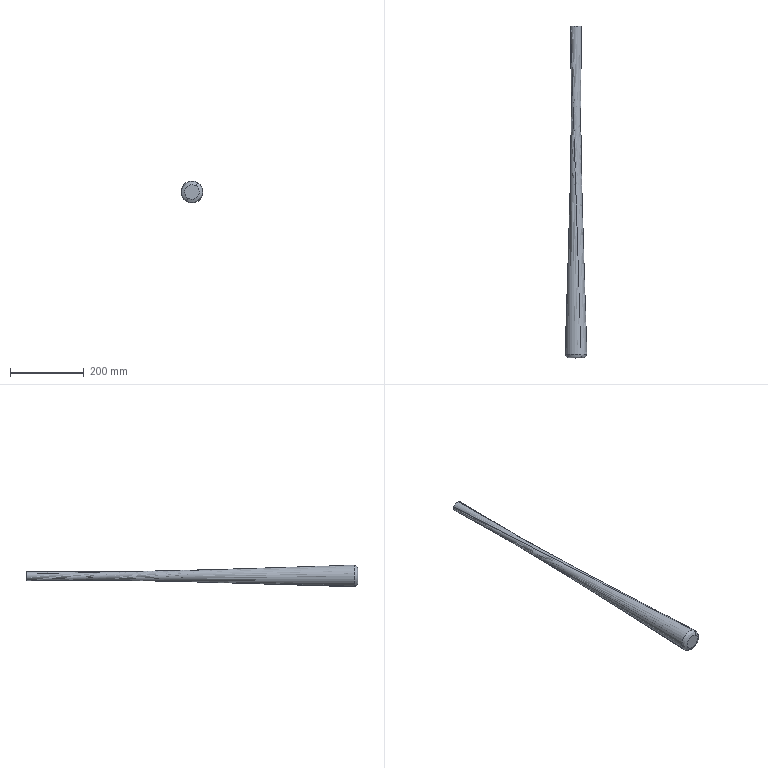Part | SolidWorks | features Blend 1, Fillet 1, RefAxis 1 | 1 solid | 6 faces | box 59.295 x 900 x 59.299 mm | volume 989144 mm3 | spline 4 | plane 2
STEP:
#1=CARTESIAN_POINT('',(-16.101,10.357,-24.873));
#2=VERTEX_POINT('',#1);
#3=CARTESIAN_POINT('',(13.223,10.355,26.518));
#4=VERTEX_POINT('',#3);
#5=CARTESIAN_POINT('',(-16.101,10.357,-24.873));
#6=CARTESIAN_POINT('',(-16.889,10.357,-24.362));
#7=CARTESIAN_POINT('',(-17.653,10.358,-23.815));
#8=CARTESIAN_POINT('',(-19.131,10.358,-22.644));
#9=CARTESIAN_POINT('',(-19.839,10.358,-22.025));
#10=CARTESIAN_POINT('',(-21.861,10.359,-20.085));
#11=CARTESIAN_POINT('',(-23.077,10.359,-18.676));
#12=CARTESIAN_POINT('',(-24.431,10.358,-16.769));
#13=CARTESIAN_POINT('',(-24.694,10.358,-16.38));
#14=CARTESIAN_POINT('',(-25.202,10.358,-15.588));
#15=CARTESIAN_POINT('',(-25.447,10.357,-15.184));
#16=CARTESIAN_POINT('',(-26.151,10.357,-13.963));
#17=CARTESIAN_POINT('',(-26.578,10.356,-13.132));
#18=CARTESIAN_POINT('',(-27.738,10.355,-10.589));
#19=CARTESIAN_POINT('',(-28.35,10.354,-8.829));
#20=CARTESIAN_POINT('',(-28.907,10.352,-6.545));
#21=CARTESIAN_POINT('',(-29.008,10.351,-6.083));
#22=CARTESIAN_POINT('',(-29.188,10.35,-5.16));
#23=CARTESIAN_POINT('',(-29.266,10.35,-4.698));
#24=CARTESIAN_POINT('',(-29.468,10.349,-3.31));
#25=CARTESIAN_POINT('',(-29.648,10.347,-1.456));
#26=CARTESIAN_POINT('',(-29.654,10.345,0.4073));
#27=CARTESIAN_POINT('',(-29.592,10.344,1.808));
#28=CARTESIAN_POINT('',(-29.56,10.344,2.275));
#29=CARTESIAN_POINT('',(-29.474,10.343,3.211));
#30=CARTESIAN_POINT('',(-29.42,10.342,3.681));
#31=CARTESIAN_POINT('',(-29.093,10.34,6.01));
#32=CARTESIAN_POINT('',(-28.659,10.339,7.823));
#33=CARTESIAN_POINT('',(-27.758,10.336,10.468));
#34=CARTESIAN_POINT('',(-27.416,10.336,11.337));
#35=CARTESIAN_POINT('',(-26.837,10.335,12.621));
#36=CARTESIAN_POINT('',(-26.633,10.334,13.047));
#37=CARTESIAN_POINT('',(-26.206,10.334,13.887));
#38=CARTESIAN_POINT('',(-25.983,10.334,14.3));
#39=CARTESIAN_POINT('',(-24.824,10.332,16.332));
#40=CARTESIAN_POINT('',(-23.753,10.332,17.855));
#41=CARTESIAN_POINT('',(-21.933,10.331,19.984));
#42=CARTESIAN_POINT('',(-21.29,10.331,20.669));
#43=CARTESIAN_POINT('',(-19.934,10.331,21.98));
#44=CARTESIAN_POINT('',(-19.23,10.331,22.597));
#45=CARTESIAN_POINT('',(-17.043,10.331,24.342));
#46=CARTESIAN_POINT('',(-15.485,10.332,25.362));
#47=CARTESIAN_POINT('',(-12.996,10.333,26.672));
#48=CARTESIAN_POINT('',(-12.138,10.334,27.073));
#49=CARTESIAN_POINT('',(-10.403,10.335,27.784));
#50=CARTESIAN_POINT('',(-9.524,10.336,28.097));
#51=CARTESIAN_POINT('',(-6.852,10.338,28.908));
#52=CARTESIAN_POINT('',(-5.025,10.339,29.281));
#53=CARTESIAN_POINT('',(-2.211,10.342,29.578));
#54=CARTESIAN_POINT('',(-1.273,10.343,29.632));
#55=CARTESIAN_POINT('',(0.5936,10.344,29.652));
#56=CARTESIAN_POINT('',(1.524,10.345,29.618));
#57=CARTESIAN_POINT('',(3.379,10.347,29.462));
#58=CARTESIAN_POINT('',(4.303,10.348,29.34));
#59=CARTESIAN_POINT('',(6.146,10.35,29.009));
#60=CARTESIAN_POINT('',(7.068,10.35,28.797));
#61=CARTESIAN_POINT('',(9.785,10.353,28.035));
#62=CARTESIAN_POINT('',(11.535,10.354,27.361));
#63=CARTESIAN_POINT('',(13.223,10.355,26.518));
#64=B_SPLINE_CURVE_WITH_KNOTS('',3,(#5,#6,#7,#8,#9,#10,#11,#12,#13,#14,#15,#16,#17,#18,#19,#20,#21,#22,#23,#24,#25,#26,#27,#28,#29,#30,#31,#32,#33,#34,#35,#36,#37,#38,#39,#40,#41,#42,#43,#44,#45,#46,#47,#48,#49,#50,#51,#52,#53,#54,#55,#56,#57,#58,#59,#60,#61,#62,#63),.UNSPECIFIED.,.F.,.F.,(4,2,2,2,2,2,2,2,2,2,1,2,2,2,2,2,2,2,2,2,2,2,2,2,2,2,2,2,2,4),(0.09701,0.09984,0.1027,0.1083,0.1097,0.1112,0.114,0.1196,0.1211,0.1225,0.1253,0.1281,0.1295,0.1309,0.1366,0.1394,0.1408,0.1423,0.1479,0.1507,0.1536,0.1592,0.1621,0.1649,0.1705,0.1734,0.1762,0.179,0.1818,0.1875),.UNSPECIFIED.);
#65=EDGE_CURVE('',#2,#4,#64,.T.);
#66=ORIENTED_EDGE('',*,*,#65,.F.);
#67=CARTESIAN_POINT('',(-10.667,0.,-16.486));
#68=VERTEX_POINT('',#67);
#69=CARTESIAN_POINT('',(-10.667,10.,-16.486));
#70=DIRECTION('',(-0.8392,0.,0.5438));
#71=DIRECTION('',(0.5438,0.,0.8392));
#72=AXIS2_PLACEMENT_3D('',#69,#70,#71);
#73=CIRCLE('',#72,10.);
#74=EDGE_CURVE('',#2,#68,#73,.T.);
#75=ORIENTED_EDGE('',*,*,#74,.T.);
#76=CARTESIAN_POINT('',(10.667,0.,16.486));
#77=VERTEX_POINT('',#76);
#78=CARTESIAN_POINT('',(10.667,0.,16.486));
#79=CARTESIAN_POINT('',(9.578,0.,17.192));
#80=CARTESIAN_POINT('',(8.42,0.,17.788));
#81=CARTESIAN_POINT('',(6.623,0.,18.501));
#82=CARTESIAN_POINT('',(6.013,0.,18.709));
#83=CARTESIAN_POINT('',(4.771,0.,19.066));
#84=CARTESIAN_POINT('',(4.137,0.,19.214));
#85=CARTESIAN_POINT('',(2.239,0.,19.561));
#86=CARTESIAN_POINT('',(0.964,0.,19.667));
#87=CARTESIAN_POINT('',(-0.9605,0.,19.638));
#88=CARTESIAN_POINT('',(-1.607,0.,19.597));
#89=CARTESIAN_POINT('',(-2.893,0.,19.451));
#90=CARTESIAN_POINT('',(-3.527,0.,19.346));
#91=CARTESIAN_POINT('',(-5.406,0.,18.943));
#92=CARTESIAN_POINT('',(-6.625,0.,18.554));
#93=CARTESIAN_POINT('',(-8.403,0.,17.786));
#94=CARTESIAN_POINT('',(-8.986,0.,17.499));
#95=CARTESIAN_POINT('',(-10.11,0.,16.875));
#96=CARTESIAN_POINT('',(-11.198,0.,16.2));
#97=CARTESIAN_POINT('',(-12.215,0.,15.422));
#98=CARTESIAN_POINT('',(-12.95,0.,14.8));
#99=CARTESIAN_POINT('',(-13.191,0.,14.586));
#100=CARTESIAN_POINT('',(-13.663,0.,14.144));
#101=CARTESIAN_POINT('',(-13.895,0.,13.917));
#102=CARTESIAN_POINT('',(-15.019,0.,12.757));
#103=CARTESIAN_POINT('',(-15.814,0.,11.754));
#104=CARTESIAN_POINT('',(-16.856,0.,10.14));
#105=CARTESIAN_POINT('',(-17.178,0.,9.584));
#106=CARTESIAN_POINT('',(-17.77,0.,8.434));
#107=CARTESIAN_POINT('',(-18.037,0.,7.843));
#108=CARTESIAN_POINT('',(-18.745,0.,6.052));
#109=CARTESIAN_POINT('',(-19.097,0.,4.823));
#110=CARTESIAN_POINT('',(-19.444,0.,2.924));
#111=CARTESIAN_POINT('',(-19.529,0.,2.279));
#112=CARTESIAN_POINT('',(-19.634,0.,0.9937));
#113=CARTESIAN_POINT('',(-19.655,0.,0.3525));
#114=CARTESIAN_POINT('',(-19.624,0.,-1.567));
#115=CARTESIAN_POINT('',(-19.48,0.,-2.84));
#116=CARTESIAN_POINT('',(-18.935,0.,-5.374));
#117=CARTESIAN_POINT('',(-18.542,0.,-6.597));
#118=CARTESIAN_POINT('',(-17.781,0.,-8.358));
#119=CARTESIAN_POINT('',(-17.498,0.,-8.934));
#120=CARTESIAN_POINT('',(-16.874,0.,-10.061));
#121=CARTESIAN_POINT('',(-16.531,0.,-10.614));
#122=CARTESIAN_POINT('',(-15.434,0.,-12.204));
#123=CARTESIAN_POINT('',(-14.608,0.,-13.181));
#124=CARTESIAN_POINT('',(-13.229,0.,-14.523));
#125=CARTESIAN_POINT('',(-12.745,0.,-14.95));
#126=CARTESIAN_POINT('',(-11.732,0.,-15.758));
#127=CARTESIAN_POINT('',(-11.208,0.,-16.135));
#128=CARTESIAN_POINT('',(-10.667,0.,-16.486));
#129=B_SPLINE_CURVE_WITH_KNOTS('',3,(#78,#79,#80,#81,#82,#83,#84,#85,#86,#87,#88,#89,#90,#91,#92,#93,#94,#95,#96,#97,#98,#99,#100,#101,#102,#103,#104,#105,#106,#107,#108,#109,#110,#111,#112,#113,#114,#115,#116,#117,#118,#119,#120,#121,#122,#123,#124,#125,#126,#127,#128),.UNSPECIFIED.,.F.,.F.,(4,2,2,2,2,2,2,2,2,1,2,2,2,2,2,2,2,2,2,2,2,2,2,2,2,4),(0.1217,0.1255,0.1275,0.1294,0.1333,0.1352,0.1371,0.141,0.1429,0.1449,0.1468,0.1478,0.1487,0.1526,0.1545,0.1565,0.1603,0.1623,0.1642,0.168,0.1719,0.1738,0.1758,0.1796,0.1816,0.1835),.UNSPECIFIED.);
#130=EDGE_CURVE('',#77,#68,#129,.T.);
#131=ORIENTED_EDGE('',*,*,#130,.F.);
#132=CARTESIAN_POINT('',(16.101,10.357,24.873));
#133=VERTEX_POINT('',#132);
#134=CARTESIAN_POINT('',(10.667,10.,16.486));
#135=DIRECTION('',(0.8392,0.,-0.5438));
#136=DIRECTION('',(-0.5438,0.,-0.8392));
#137=AXIS2_PLACEMENT_3D('',#134,#135,#136);
#138=CIRCLE('',#137,10.);
#139=EDGE_CURVE('',#133,#77,#138,.T.);
#140=ORIENTED_EDGE('',*,*,#139,.F.);
#141=CARTESIAN_POINT('',(13.223,10.355,26.518));
#142=CARTESIAN_POINT('',(13.717,10.356,26.271));
#143=CARTESIAN_POINT('',(14.205,10.356,26.01));
#144=CARTESIAN_POINT('',(15.165,10.356,25.461));
#145=CARTESIAN_POINT('',(15.637,10.357,25.174));
#146=CARTESIAN_POINT('',(16.101,10.357,24.873));
#147=B_SPLINE_CURVE_WITH_KNOTS('',3,(#141,#142,#143,#144,#145,#146),.UNSPECIFIED.,.F.,.F.,(4,2,4),(0.1875,0.1892,0.1908),.UNSPECIFIED.);
#148=EDGE_CURVE('',#4,#133,#147,.T.);
#149=ORIENTED_EDGE('',*,*,#148,.F.);
#150=EDGE_LOOP('',(#66,#75,#131,#140,#149));
#151=FACE_OUTER_BOUND('',#150,.T.);
#152=CARTESIAN_POINT('',(16.101,10.357,24.873));
#153=CARTESIAN_POINT('',(16.302,0.,25.183));
#154=CARTESIAN_POINT('',(10.667,0.,16.486));
#155=CARTESIAN_POINT('',(14.459,10.356,25.937));
#156=CARTESIAN_POINT('',(14.639,0.,26.26));
#157=CARTESIAN_POINT('',(9.577,0.,17.192));
#158=CARTESIAN_POINT('',(12.74,10.355,26.823));
#159=CARTESIAN_POINT('',(12.898,0.,27.156));
#160=CARTESIAN_POINT('',(8.437,0.,17.78));
#161=CARTESIAN_POINT('',(10.05,10.353,27.895));
#162=CARTESIAN_POINT('',(10.174,0.,28.239));
#163=CARTESIAN_POINT('',(6.653,0.,18.49));
#164=CARTESIAN_POINT('',(9.135,10.352,28.209));
#165=CARTESIAN_POINT('',(9.247,0.,28.556));
#166=CARTESIAN_POINT('',(6.046,0.,18.698));
#167=CARTESIAN_POINT('',(7.266,10.351,28.749));
#168=CARTESIAN_POINT('',(7.355,0.,29.101));
#169=CARTESIAN_POINT('',(4.807,0.,19.056));
#170=CARTESIAN_POINT('',(6.31,10.35,28.974));
#171=CARTESIAN_POINT('',(6.387,0.,29.328));
#172=CARTESIAN_POINT('',(4.173,0.,19.206));
#173=CARTESIAN_POINT('',(3.444,10.347,29.504));
#174=CARTESIAN_POINT('',(3.486,0.,29.861));
#175=CARTESIAN_POINT('',(2.273,0.,19.557));
#176=CARTESIAN_POINT('',(1.52,10.345,29.667));
#177=CARTESIAN_POINT('',(1.539,0.,30.024));
#178=CARTESIAN_POINT('',(0.998,0.,19.665));
#179=CARTESIAN_POINT('',(-0.9007,10.343,29.635));
#180=CARTESIAN_POINT('',(-0.9112,0.,29.99));
#181=CARTESIAN_POINT('',(-0.6067,0.,19.644));
#182=CARTESIAN_POINT('',(-1.386,10.343,29.617));
#183=CARTESIAN_POINT('',(-1.402,0.,29.971));
#184=CARTESIAN_POINT('',(-0.9282,0.,19.632));
#185=CARTESIAN_POINT('',(-2.358,10.342,29.556));
#186=CARTESIAN_POINT('',(-2.385,0.,29.909));
#187=CARTESIAN_POINT('',(-1.572,0.,19.592));
#188=CARTESIAN_POINT('',(-2.846,10.341,29.514));
#189=CARTESIAN_POINT('',(-2.879,0.,29.865));
#190=CARTESIAN_POINT('',(-1.896,0.,19.563));
#191=CARTESIAN_POINT('',(-4.303,10.34,29.35));
#192=CARTESIAN_POINT('',(-4.354,0.,29.699));
#193=CARTESIAN_POINT('',(-2.861,0.,19.455));
#194=CARTESIAN_POINT('',(-5.261,10.339,29.194));
#195=CARTESIAN_POINT('',(-5.323,0.,29.54));
#196=CARTESIAN_POINT('',(-3.497,0.,19.352));
#197=CARTESIAN_POINT('',(-8.099,10.337,28.589));
#198=CARTESIAN_POINT('',(-8.194,0.,28.925));
#199=CARTESIAN_POINT('',(-5.377,0.,18.951));
#200=CARTESIAN_POINT('',(-9.942,10.335,28.005));
#201=CARTESIAN_POINT('',(-10.058,0.,28.332));
#202=CARTESIAN_POINT('',(-6.598,0.,18.563));
#203=CARTESIAN_POINT('',(-12.181,10.334,27.042));
#204=CARTESIAN_POINT('',(-12.322,0.,27.357));
#205=CARTESIAN_POINT('',(-8.081,0.,17.925));
#206=CARTESIAN_POINT('',(-12.627,10.334,26.837));
#207=CARTESIAN_POINT('',(-12.773,0.,27.149));
#208=CARTESIAN_POINT('',(-8.376,0.,17.79));
#209=CARTESIAN_POINT('',(-13.504,10.333,26.407));
#210=CARTESIAN_POINT('',(-13.661,0.,26.713));
#211=CARTESIAN_POINT('',(-8.957,0.,17.505));
#212=CARTESIAN_POINT('',(-13.936,10.333,26.182));
#213=CARTESIAN_POINT('',(-14.097,0.,26.486));
#214=CARTESIAN_POINT('',(-9.243,0.,17.356));
#215=CARTESIAN_POINT('',(-15.21,10.332,25.477));
#216=CARTESIAN_POINT('',(-15.386,0.,25.772));
#217=CARTESIAN_POINT('',(-10.088,0.,16.889));
#218=CARTESIAN_POINT('',(-16.033,10.332,24.968));
#219=CARTESIAN_POINT('',(-16.218,0.,25.257));
#220=CARTESIAN_POINT('',(-10.632,0.,16.552));
#221=CARTESIAN_POINT('',(-17.624,10.331,23.872));
#222=CARTESIAN_POINT('',(-17.827,0.,24.148));
#223=CARTESIAN_POINT('',(-11.686,0.,15.826));
#224=CARTESIAN_POINT('',(-18.393,10.331,23.286));
#225=CARTESIAN_POINT('',(-18.605,0.,23.554));
#226=CARTESIAN_POINT('',(-12.195,0.,15.437));
#227=CARTESIAN_POINT('',(-19.505,10.331,22.347));
#228=CARTESIAN_POINT('',(-19.73,0.,22.604));
#229=CARTESIAN_POINT('',(-12.932,0.,14.815));
#230=CARTESIAN_POINT('',(-19.868,10.331,22.024));
#231=CARTESIAN_POINT('',(-20.098,0.,22.278));
#232=CARTESIAN_POINT('',(-13.173,0.,14.602));
#233=CARTESIAN_POINT('',(-20.582,10.331,21.358));
#234=CARTESIAN_POINT('',(-20.82,0.,21.605));
#235=CARTESIAN_POINT('',(-13.646,0.,14.161));
#236=CARTESIAN_POINT('',(-20.933,10.331,21.015));
#237=CARTESIAN_POINT('',(-21.174,0.,21.257));
#238=CARTESIAN_POINT('',(-13.878,0.,13.933));
#239=CARTESIAN_POINT('',(-22.633,10.331,19.264));
#240=CARTESIAN_POINT('',(-22.895,0.,19.486));
#241=CARTESIAN_POINT('',(-15.004,0.,12.774));
#242=CARTESIAN_POINT('',(-23.837,10.332,17.75));
#243=CARTESIAN_POINT('',(-24.113,0.,17.955));
#244=CARTESIAN_POINT('',(-15.802,0.,11.771));
#245=CARTESIAN_POINT('',(-25.414,10.333,15.314));
#246=CARTESIAN_POINT('',(-25.709,0.,15.492));
#247=CARTESIAN_POINT('',(-16.846,0.,10.157));
#248=CARTESIAN_POINT('',(-25.901,10.334,14.474));
#249=CARTESIAN_POINT('',(-26.202,0.,14.642));
#250=CARTESIAN_POINT('',(-17.169,0.,9.601));
#251=CARTESIAN_POINT('',(-26.572,10.334,13.172));
#252=CARTESIAN_POINT('',(-26.882,0.,13.325));
#253=CARTESIAN_POINT('',(-17.614,0.,8.738));
#254=CARTESIAN_POINT('',(-26.786,10.335,12.73));
#255=CARTESIAN_POINT('',(-27.099,0.,12.879));
#256=CARTESIAN_POINT('',(-17.755,0.,8.446));
#257=CARTESIAN_POINT('',(-27.19,10.335,11.843));
#258=CARTESIAN_POINT('',(-27.508,0.,11.981));
#259=CARTESIAN_POINT('',(-18.023,0.,7.858));
#260=CARTESIAN_POINT('',(-27.38,10.336,11.395));
#261=CARTESIAN_POINT('',(-27.7,0.,11.529));
#262=CARTESIAN_POINT('',(-18.148,0.,7.561));
#263=CARTESIAN_POINT('',(-28.273,10.337,9.142));
#264=CARTESIAN_POINT('',(-28.605,0.,9.249));
#265=CARTESIAN_POINT('',(-18.74,0.,6.068));
#266=CARTESIAN_POINT('',(-28.805,10.339,7.286));
#267=CARTESIAN_POINT('',(-29.146,0.,7.371));
#268=CARTESIAN_POINT('',(-19.093,0.,4.838));
#269=CARTESIAN_POINT('',(-29.243,10.341,4.898));
#270=CARTESIAN_POINT('',(-29.591,0.,4.956));
#271=CARTESIAN_POINT('',(-19.383,0.,3.256));
#272=CARTESIAN_POINT('',(-29.319,10.342,4.417));
#273=CARTESIAN_POINT('',(-29.669,0.,4.469));
#274=CARTESIAN_POINT('',(-19.434,0.,2.937));
#275=CARTESIAN_POINT('',(-29.448,10.343,3.448));
#276=CARTESIAN_POINT('',(-29.8,0.,3.489));
#277=CARTESIAN_POINT('',(-19.519,0.,2.295));
#278=CARTESIAN_POINT('',(-29.5,10.343,2.961));
#279=CARTESIAN_POINT('',(-29.854,0.,2.996));
#280=CARTESIAN_POINT('',(-19.554,0.,1.972));
#281=CARTESIAN_POINT('',(-29.621,10.344,1.505));
#282=CARTESIAN_POINT('',(-29.977,0.,1.523));
#283=CARTESIAN_POINT('',(-19.634,0.,1.007));
#284=CARTESIAN_POINT('',(-29.653,10.345,0.5371));
#285=CARTESIAN_POINT('',(-30.011,0.,0.5432));
#286=CARTESIAN_POINT('',(-19.655,0.,0.3657));
#287=CARTESIAN_POINT('',(-29.608,10.348,-2.36));
#288=CARTESIAN_POINT('',(-29.968,0.,-2.389));
#289=CARTESIAN_POINT('',(-19.625,0.,-1.555));
#290=CARTESIAN_POINT('',(-29.392,10.35,-4.282));
#291=CARTESIAN_POINT('',(-29.751,0.,-4.334));
#292=CARTESIAN_POINT('',(-19.482,0.,-2.829));
#293=CARTESIAN_POINT('',(-28.776,10.352,-7.15));
#294=CARTESIAN_POINT('',(-29.13,0.,-7.239));
#295=CARTESIAN_POINT('',(-19.074,0.,-4.731));
#296=CARTESIAN_POINT('',(-28.524,10.353,-8.091));
#297=CARTESIAN_POINT('',(-28.876,0.,-8.191));
#298=CARTESIAN_POINT('',(-18.907,0.,-5.355));
#299=CARTESIAN_POINT('',(-27.934,10.354,-9.934));
#300=CARTESIAN_POINT('',(-28.28,0.,-10.058));
#301=CARTESIAN_POINT('',(-18.516,0.,-6.577));
#302=CARTESIAN_POINT('',(-27.596,10.355,-10.838));
#303=CARTESIAN_POINT('',(-27.938,0.,-10.973));
#304=CARTESIAN_POINT('',(-18.291,0.,-7.177));
#305=CARTESIAN_POINT('',(-26.831,10.356,-12.61));
#306=CARTESIAN_POINT('',(-27.165,0.,-12.767));
#307=CARTESIAN_POINT('',(-17.784,0.,-8.352));
#308=CARTESIAN_POINT('',(-26.405,10.357,-13.478));
#309=CARTESIAN_POINT('',(-26.734,0.,-13.646));
#310=CARTESIAN_POINT('',(-17.501,0.,-8.928));
#311=CARTESIAN_POINT('',(-25.464,10.357,-15.179));
#312=CARTESIAN_POINT('',(-25.783,0.,-15.369));
#313=CARTESIAN_POINT('',(-16.878,0.,-10.056));
#314=CARTESIAN_POINT('',(-24.947,10.358,-16.014));
#315=CARTESIAN_POINT('',(-25.259,0.,-16.215));
#316=CARTESIAN_POINT('',(-16.534,0.,-10.61));
#317=CARTESIAN_POINT('',(-23.293,10.359,-18.413));
#318=CARTESIAN_POINT('',(-23.585,0.,-18.644));
#319=CARTESIAN_POINT('',(-15.437,0.,-12.201));
#320=CARTESIAN_POINT('',(-22.047,10.359,-19.886));
#321=CARTESIAN_POINT('',(-22.324,0.,-20.136));
#322=CARTESIAN_POINT('',(-14.611,0.,-13.178));
#323=CARTESIAN_POINT('',(-19.967,10.359,-21.91));
#324=CARTESIAN_POINT('',(-20.218,0.,-22.185));
#325=CARTESIAN_POINT('',(-13.231,0.,-14.521));
#326=CARTESIAN_POINT('',(-19.237,10.358,-22.555));
#327=CARTESIAN_POINT('',(-19.478,0.,-22.838));
#328=CARTESIAN_POINT('',(-12.747,0.,-14.949));
#329=CARTESIAN_POINT('',(-17.708,10.358,-23.775));
#330=CARTESIAN_POINT('',(-17.93,0.,-24.072));
#331=CARTESIAN_POINT('',(-11.733,0.,-15.758));
#332=CARTESIAN_POINT('',(-16.918,10.357,-24.344));
#333=CARTESIAN_POINT('',(-17.13,0.,-24.648));
#334=CARTESIAN_POINT('',(-11.208,0.,-16.135));
#335=CARTESIAN_POINT('',(-16.101,10.357,-24.873));
#336=CARTESIAN_POINT('',(-16.302,0.,-25.183));
#337=CARTESIAN_POINT('',(-10.667,0.,-16.486));
#338=(BOUNDED_SURFACE()B_SPLINE_SURFACE(3,2,((#152,#153,#154),(#155,#156,#157),(#158,#159,#160),(#161,#162,#163),(#164,#165,#166),(#167,#168,#169),(#170,#171,#172),(#173,#174,#175),(#176,#177,#178),(#179,#180,#181),(#182,#183,#184),(#185,#186,#187),(#188,#189,#190),(#191,#192,#193),(#194,#195,#196),(#197,#198,#199),(#200,#201,#202),(#203,#204,#205),(#206,#207,#208),(#209,#210,#211),(#212,#213,#214),(#215,#216,#217),(#218,#219,#220),(#221,#222,#223),(#224,#225,#226),(#227,#228,#229),(#230,#231,#232),(#233,#234,#235),(#236,#237,#238),(#239,#240,#241),(#242,#243,#244),(#245,#246,#247),(#248,#249,#250),(#251,#252,#253),(#254,#255,#256),(#257,#258,#259),(#260,#261,#262),(#263,#264,#265),(#266,#267,#268),(#269,#270,#271),(#272,#273,#274),(#275,#276,#277),(#278,#279,#280),(#281,#282,#283),(#284,#285,#286),(#287,#288,#289),(#290,#291,#292),(#293,#294,#295),(#296,#297,#298),(#299,#300,#301),(#302,#303,#304),(#305,#306,#307),(#308,#309,#310),(#311,#312,#313),(#314,#315,#316),(#317,#318,#319),(#320,#321,#322),(#323,#324,#325),(#326,#327,#328),(#329,#330,#331),(#332,#333,#334),(#335,#336,#337)),.UNSPECIFIED.,.F.,.F.,.F.)B_SPLINE_SURFACE_WITH_KNOTS((4,2,2,2,2,2,2,2,2,2,2,2,2,2,2,2,2,2,2,2,2,2,2,2,2,2,2,2,2,2,4),(3,3),(0.,0.003839,0.005758,0.007678,0.01152,0.01248,0.01344,0.01536,0.01919,0.02015,0.02111,0.02303,0.02495,0.02591,0.02687,0.03071,0.03263,0.03359,0.03455,0.03839,0.03935,0.04031,0.04223,0.04607,0.04799,0.0499,0.05182,0.05374,0.05758,0.0595,0.06142),(0.,1.),.UNSPECIFIED.)GEOMETRIC_REPRESENTATION_ITEM()RATIONAL_B_SPLINE_SURFACE(((1.,0.6944,1.),(1.,0.6944,1.),(1.,0.6944,1.),(1.,0.6945,1.),(1.,0.6945,1.),(1.,0.6946,1.),(1.,0.6946,1.),(1.,0.6947,1.),(1.,0.6948,1.),(1.,0.6949,1.),(1.,0.6949,1.),(1.,0.6949,1.),(1.,0.6949,1.),(1.,0.695,1.),(1.,0.695,1.),(1.,0.6951,1.),(1.,0.6952,1.),(1.,0.6952,1.),(1.,0.6952,1.),(1.,0.6952,1.),(1.,0.6952,1.),(1.,0.6953,1.),(1.,0.6953,1.),(1.,0.6953,1.),(1.,0.6953,1.),(1.,0.6953,1.),(1.,0.6953,1.),(1.,0.6953,1.),(1.,0.6953,1.),(1.,0.6953,1.),(1.,0.6953,1.),(1.,0.6952,1.),(1.,0.6952,1.),(1.,0.6952,1.),(1.,0.6952,1.),(1.,0.6951,1.),(1.,0.6951,1.),(1.,0.6951,1.),(1.,0.695,1.),(1.,0.6949,1.),(1.,0.6949,1.),(1.,0.6949,1.),(1.,0.6949,1.),(1.,0.6948,1.),(1.,0.6948,1.),(1.,0.6947,1.),(1.,0.6946,1.),(1.,0.6945,1.),(1.,0.6945,1.),(1.,0.6945,1.),(1.,0.6944,1.),(1.,0.6944,1.),(1.,0.6944,1.),(1.,0.6944,1.),(1.,0.6943,1.),(1.,0.6943,1.),(1.,0.6943,1.),(1.,0.6943,1.),(1.,0.6943,1.),(1.,0.6943,1.),(1.,0.6944,1.),(1.,0.6944,1.)))REPRESENTATION_ITEM('')SURFACE());
#339=ADVANCED_FACE('',(#151),#338,.T.);
#340=CARTESIAN_POINT('',(13.894,900.,-4.711));
#341=VERTEX_POINT('',#340);
#342=CARTESIAN_POINT('',(-13.894,900.,4.711));
#343=VERTEX_POINT('',#342);
#344=CARTESIAN_POINT('',(13.894,900.,-4.711));
#345=CARTESIAN_POINT('',(2.588,900.,-27.868));
#346=CARTESIAN_POINT('',(-25.2,900.,-18.446));
#347=CARTESIAN_POINT('',(-13.894,900.,4.711));
#348=(BOUNDED_CURVE()B_SPLINE_CURVE(3,(#344,#345,#346,#347),.UNSPECIFIED.,.F.,.F.)B_SPLINE_CURVE_WITH_KNOTS((4,4),(0.3864,3.528),.UNSPECIFIED.)CURVE()GEOMETRIC_REPRESENTATION_ITEM()RATIONAL_B_SPLINE_CURVE((1.,0.3333,0.3333,1.))REPRESENTATION_ITEM(''));
#349=EDGE_CURVE('',#341,#343,#348,.T.);
#350=ORIENTED_EDGE('',*,*,#349,.F.);
#351=CARTESIAN_POINT('',(-13.223,10.355,-26.518));
#352=VERTEX_POINT('',#351);
#353=CARTESIAN_POINT('',(13.894,900.,-4.711));
#354=CARTESIAN_POINT('',(-13.223,10.355,-26.518));
#355=B_SPLINE_CURVE_WITH_KNOTS('',1,(#353,#354),.UNSPECIFIED.,.F.,.F.,(2,2),(0.,0.9885),.UNSPECIFIED.);
#356=EDGE_CURVE('',#341,#352,#355,.T.);
#357=ORIENTED_EDGE('',*,*,#356,.T.);
#358=CARTESIAN_POINT('',(-13.223,10.355,-26.518));
#359=CARTESIAN_POINT('',(-13.719,10.356,-26.27));
#360=CARTESIAN_POINT('',(-14.207,10.356,-26.008));
#361=CARTESIAN_POINT('',(-15.167,10.356,-25.46));
#362=CARTESIAN_POINT('',(-15.638,10.357,-25.173));
#363=CARTESIAN_POINT('',(-16.101,10.357,-24.873));
#364=B_SPLINE_CURVE_WITH_KNOTS('',3,(#358,#359,#360,#361,#362,#363),.UNSPECIFIED.,.F.,.F.,(4,2,4),(0.09369,0.09535,0.09701),.UNSPECIFIED.);
#365=EDGE_CURVE('',#352,#2,#364,.T.);
#366=ORIENTED_EDGE('',*,*,#365,.T.);
#367=ORIENTED_EDGE('',*,*,#65,.T.);
#368=CARTESIAN_POINT('',(-13.894,900.,4.711));
#369=CARTESIAN_POINT('',(13.223,10.355,26.518));
#370=B_SPLINE_CURVE_WITH_KNOTS('',1,(#368,#369),.UNSPECIFIED.,.F.,.F.,(2,2),(0.,0.9885),.UNSPECIFIED.);
#371=EDGE_CURVE('',#343,#4,#370,.T.);
#372=ORIENTED_EDGE('',*,*,#371,.F.);
#373=EDGE_LOOP('',(#350,#357,#366,#367,#372));
#374=FACE_OUTER_BOUND('',#373,.T.);
#375=CARTESIAN_POINT('',(-13.894,900.,4.711));
#376=CARTESIAN_POINT('',(13.538,0.,26.772));
#377=CARTESIAN_POINT('',(-25.2,900.,-18.446));
#378=CARTESIAN_POINT('',(-40.005,0.,53.848));
#379=CARTESIAN_POINT('',(2.588,900.,-27.868));
#380=CARTESIAN_POINT('',(-67.081,0.,0.3051));
#381=CARTESIAN_POINT('',(13.894,900.,-4.711));
#382=CARTESIAN_POINT('',(-13.538,0.,-26.772));
#383=CARTESIAN_POINT('',(25.2,900.,18.446));
#384=CARTESIAN_POINT('',(40.005,0.,-53.848));
#385=CARTESIAN_POINT('',(-2.588,900.,27.868));
#386=CARTESIAN_POINT('',(67.081,0.,-0.3051));
#387=CARTESIAN_POINT('',(-13.894,900.,4.711));
#388=CARTESIAN_POINT('',(13.538,0.,26.772));
#389=(BOUNDED_SURFACE()B_SPLINE_SURFACE(3,1,((#375,#376),(#377,#378),(#379,#380),(#381,#382),(#383,#384),(#385,#386),(#387,#388)),.UNSPECIFIED.,.T.,.F.,.T.)B_SPLINE_SURFACE_WITH_KNOTS((4,3,4),(2,2),(0.,0.5,1.),(0.,1.),.UNSPECIFIED.)GEOMETRIC_REPRESENTATION_ITEM()RATIONAL_B_SPLINE_SURFACE(((1.,1.),(0.3333,0.3333),(0.3333,0.3333),(1.,1.),(0.3333,0.3333),(0.3333,0.3333),(1.,1.)))REPRESENTATION_ITEM('')SURFACE());
#390=ADVANCED_FACE('',(#374),#389,.T.);
#391=ORIENTED_EDGE('',*,*,#130,.T.);
#392=CARTESIAN_POINT('',(-10.667,0.,-16.486));
#393=CARTESIAN_POINT('',(-10.125,0.,-16.837));
#394=CARTESIAN_POINT('',(-9.566,0.,-17.162));
#395=CARTESIAN_POINT('',(-8.414,0.,-17.756));
#396=CARTESIAN_POINT('',(-7.825,0.,-18.024));
#397=CARTESIAN_POINT('',(-6.036,0.,-18.735));
#398=CARTESIAN_POINT('',(-4.806,0.,-19.089));
#399=CARTESIAN_POINT('',(-2.905,0.,-19.44));
#400=CARTESIAN_POINT('',(-2.26,0.,-19.527));
#401=CARTESIAN_POINT('',(-0.9751,0.,-19.635));
#402=CARTESIAN_POINT('',(-0.334,0.,-19.657));
#403=CARTESIAN_POINT('',(1.586,0.,-19.63));
#404=CARTESIAN_POINT('',(2.863,0.,-19.487));
#405=CARTESIAN_POINT('',(5.4,0.,-18.945));
#406=CARTESIAN_POINT('',(6.621,0.,-18.554));
#407=CARTESIAN_POINT('',(8.385,0.,-17.794));
#408=CARTESIAN_POINT('',(8.961,0.,-17.512));
#409=CARTESIAN_POINT('',(10.091,0.,-16.887));
#410=CARTESIAN_POINT('',(10.644,0.,-16.544));
#411=CARTESIAN_POINT('',(12.233,0.,-15.448));
#412=CARTESIAN_POINT('',(13.21,0.,-14.621));
#413=CARTESIAN_POINT('',(14.553,0.,-13.239));
#414=CARTESIAN_POINT('',(14.981,0.,-12.752));
#415=CARTESIAN_POINT('',(15.787,0.,-11.738));
#416=CARTESIAN_POINT('',(16.162,0.,-11.216));
#417=CARTESIAN_POINT('',(17.204,0.,-9.601));
#418=CARTESIAN_POINT('',(17.792,0.,-8.463));
#419=CARTESIAN_POINT('',(18.387,0.,-6.96));
#420=CARTESIAN_POINT('',(18.499,0.,-6.655));
#421=CARTESIAN_POINT('',(18.707,0.,-6.043));
#422=CARTESIAN_POINT('',(18.803,0.,-5.735));
#423=CARTESIAN_POINT('',(19.068,0.,-4.808));
#424=CARTESIAN_POINT('',(19.359,0.,-3.56));
#425=CARTESIAN_POINT('',(19.528,0.,-2.29));
#426=CARTESIAN_POINT('',(19.634,0.,-1.008));
#427=CARTESIAN_POINT('',(19.655,0.,-0.3579));
#428=CARTESIAN_POINT('',(19.624,0.,1.58));
#429=CARTESIAN_POINT('',(19.478,0.,2.852));
#430=CARTESIAN_POINT('',(19.073,0.,4.732));
#431=CARTESIAN_POINT('',(18.908,0.,5.354));
#432=CARTESIAN_POINT('',(18.512,0.,6.587));
#433=CARTESIAN_POINT('',(18.284,0.,7.193));
#434=CARTESIAN_POINT('',(17.52,0.,8.961));
#435=CARTESIAN_POINT('',(16.899,0.,10.08));
#436=CARTESIAN_POINT('',(15.803,0.,11.671));
#437=CARTESIAN_POINT('',(15.407,0.,12.188));
#438=CARTESIAN_POINT('',(14.574,0.,13.173));
#439=CARTESIAN_POINT('',(14.136,0.,13.642));
#440=CARTESIAN_POINT('',(12.758,0.,14.98));
#441=CARTESIAN_POINT('',(11.756,0.,15.78));
#442=CARTESIAN_POINT('',(10.667,0.,16.486));
#443=B_SPLINE_CURVE_WITH_KNOTS('',3,(#392,#393,#394,#395,#396,#397,#398,#399,#400,#401,#402,#403,#404,#405,#406,#407,#408,#409,#410,#411,#412,#413,#414,#415,#416,#417,#418,#419,#420,#421,#422,#423,#424,#425,#426,#427,#428,#429,#430,#431,#432,#433,#434,#435,#436,#437,#438,#439,#440,#441,#442),.UNSPECIFIED.,.F.,.F.,(4,2,2,2,2,2,2,2,2,2,2,2,2,2,2,2,1,2,2,2,2,2,2,2,2,4),(0.05977,0.06171,0.06364,0.06751,0.06944,0.07138,0.07524,0.07911,0.08105,0.08298,0.08685,0.08878,0.09072,0.09459,0.09555,0.09652,0.09845,0.1004,0.1023,0.1062,0.1081,0.1101,0.1139,0.1159,0.1178,0.1217),.UNSPECIFIED.);
#444=EDGE_CURVE('',#68,#77,#443,.T.);
#445=ORIENTED_EDGE('',*,*,#444,.T.);
#446=EDGE_LOOP('',(#391,#445));
#447=FACE_OUTER_BOUND('',#446,.T.);
#448=CARTESIAN_POINT('',(0.,0.,0.));
#449=DIRECTION('',(0.,1.,0.));
#450=DIRECTION('',(0.,0.,1.));
#451=AXIS2_PLACEMENT_3D('',#448,#449,#450);
#452=PLANE('',#451);
#453=ADVANCED_FACE('',(#447),#452,.F.);
#454=CARTESIAN_POINT('',(-13.894,900.,4.711));
#455=CARTESIAN_POINT('',(-2.588,900.,27.868));
#456=CARTESIAN_POINT('',(25.2,900.,18.446));
#457=CARTESIAN_POINT('',(13.894,900.,-4.711));
#458=(BOUNDED_CURVE()B_SPLINE_CURVE(3,(#454,#455,#456,#457),.UNSPECIFIED.,.F.,.T.)B_SPLINE_CURVE_WITH_KNOTS((4,4),(3.528,6.67),.UNSPECIFIED.)CURVE()GEOMETRIC_REPRESENTATION_ITEM()RATIONAL_B_SPLINE_CURVE((1.,0.3333,0.3333,1.))REPRESENTATION_ITEM(''));
#459=EDGE_CURVE('',#343,#341,#458,.T.);
#460=ORIENTED_EDGE('',*,*,#459,.T.);
#461=ORIENTED_EDGE('',*,*,#349,.T.);
#462=EDGE_LOOP('',(#460,#461));
#463=FACE_OUTER_BOUND('',#462,.T.);
#464=CARTESIAN_POINT('',(0.,900.,0.));
#465=DIRECTION('',(0.,1.,0.));
#466=DIRECTION('',(0.,0.,1.));
#467=AXIS2_PLACEMENT_3D('',#464,#465,#466);
#468=PLANE('',#467);
#469=ADVANCED_FACE('',(#463),#468,.T.);
#470=ORIENTED_EDGE('',*,*,#356,.F.);
#471=ORIENTED_EDGE('',*,*,#459,.F.);
#472=ORIENTED_EDGE('',*,*,#371,.T.);
#473=ORIENTED_EDGE('',*,*,#148,.T.);
#474=CARTESIAN_POINT('',(16.101,10.357,24.873));
#475=CARTESIAN_POINT('',(17.686,10.358,23.846));
#476=CARTESIAN_POINT('',(19.149,10.358,22.685));
#477=CARTESIAN_POINT('',(21.166,10.359,20.752));
#478=CARTESIAN_POINT('',(21.809,10.359,20.076));
#479=CARTESIAN_POINT('',(23.035,10.359,18.657));
#480=CARTESIAN_POINT('',(23.62,10.358,17.911));
#481=CARTESIAN_POINT('',(25.25,10.358,15.615));
#482=CARTESIAN_POINT('',(26.18,10.357,14.001));
#483=CARTESIAN_POINT('',(27.343,10.355,11.455));
#484=CARTESIAN_POINT('',(27.692,10.355,10.586));
#485=CARTESIAN_POINT('',(28.156,10.354,9.251));
#486=CARTESIAN_POINT('',(28.3,10.353,8.801));
#487=CARTESIAN_POINT('',(28.566,10.353,7.899));
#488=CARTESIAN_POINT('',(28.687,10.352,7.447));
#489=CARTESIAN_POINT('',(29.241,10.351,5.177));
#490=CARTESIAN_POINT('',(29.51,10.349,3.334));
#491=CARTESIAN_POINT('',(29.627,10.347,0.9972));
#492=CARTESIAN_POINT('',(29.64,10.346,0.5281));
#493=CARTESIAN_POINT('',(29.643,10.345,-0.4136));
#494=CARTESIAN_POINT('',(29.633,10.345,-0.8866));
#495=CARTESIAN_POINT('',(29.57,10.344,-2.295));
#496=CARTESIAN_POINT('',(29.483,10.343,-3.226));
#497=CARTESIAN_POINT('',(29.095,10.34,-5.995));
#498=CARTESIAN_POINT('',(28.664,10.339,-7.809));
#499=CARTESIAN_POINT('',(27.905,10.337,-10.036));
#500=CARTESIAN_POINT('',(27.742,10.336,-10.48));
#501=CARTESIAN_POINT('',(27.396,10.336,-11.355));
#502=CARTESIAN_POINT('',(27.213,10.335,-11.787));
#503=CARTESIAN_POINT('',(26.636,10.334,-13.066));
#504=CARTESIAN_POINT('',(25.79,10.333,-14.728));
#505=CARTESIAN_POINT('',(24.791,10.332,-16.302));
#506=CARTESIAN_POINT('',(23.984,10.332,-17.449));
#507=CARTESIAN_POINT('',(23.706,10.332,-17.826));
#508=CARTESIAN_POINT('',(23.129,10.332,-18.569));
#509=CARTESIAN_POINT('',(22.83,10.331,-18.935));
#510=CARTESIAN_POINT('',(21.299,10.331,-20.723));
#511=CARTESIAN_POINT('',(19.957,10.331,-22.018));
#512=CARTESIAN_POINT('',(17.771,10.331,-23.761));
#513=CARTESIAN_POINT('',(17.014,10.331,-24.309));
#514=CARTESIAN_POINT('',(15.835,10.332,-25.08));
#515=CARTESIAN_POINT('',(15.433,10.332,-25.329));
#516=CARTESIAN_POINT('',(14.62,10.332,-25.806));
#517=CARTESIAN_POINT('',(14.21,10.333,-26.034));
#518=CARTESIAN_POINT('',(12.136,10.334,-27.122));
#519=CARTESIAN_POINT('',(10.413,10.335,-27.828));
#520=CARTESIAN_POINT('',(7.731,10.337,-28.641));
#521=CARTESIAN_POINT('',(6.819,10.338,-28.871));
#522=CARTESIAN_POINT('',(4.97,10.339,-29.244));
#523=CARTESIAN_POINT('',(4.043,10.34,-29.386));
#524=CARTESIAN_POINT('',(1.259,10.343,-29.677));
#525=CARTESIAN_POINT('',(-0.6038,10.344,-29.696));
#526=CARTESIAN_POINT('',(-3.408,10.347,-29.459));
#527=CARTESIAN_POINT('',(-4.348,10.348,-29.334));
#528=CARTESIAN_POINT('',(-6.193,10.35,-28.998));
#529=CARTESIAN_POINT('',(-7.103,10.35,-28.788));
#530=CARTESIAN_POINT('',(-9.793,10.353,-28.031));
#531=CARTESIAN_POINT('',(-11.534,10.354,-27.361));
#532=CARTESIAN_POINT('',(-13.223,10.355,-26.518));
#533=B_SPLINE_CURVE_WITH_KNOTS('',3,(#474,#475,#476,#477,#478,#479,#480,#481,#482,#483,#484,#485,#486,#487,#488,#489,#490,#491,#492,#493,#494,#495,#496,#497,#498,#499,#500,#501,#502,#503,#504,#505,#506,#507,#508,#509,#510,#511,#512,#513,#514,#515,#516,#517,#518,#519,#520,#521,#522,#523,#524,#525,#526,#527,#528,#529,#530,#531,#532),.UNSPECIFIED.,.F.,.F.,(4,2,2,2,2,2,2,2,2,2,2,2,2,2,2,1,2,2,2,2,2,2,2,2,2,2,2,2,2,4),(0.003148,0.008807,0.01164,0.01447,0.02013,0.02295,0.02437,0.02578,0.03144,0.03286,0.03427,0.0371,0.04276,0.04418,0.04559,0.04842,0.05125,0.05266,0.05408,0.05974,0.06257,0.06398,0.0654,0.07106,0.07388,0.07671,0.08237,0.0852,0.08803,0.09369),.UNSPECIFIED.);
#534=EDGE_CURVE('',#133,#352,#533,.T.);
#535=ORIENTED_EDGE('',*,*,#534,.T.);
#536=EDGE_LOOP('',(#470,#471,#472,#473,#535));
#537=FACE_OUTER_BOUND('',#536,.T.);
#538=CARTESIAN_POINT('',(-13.894,900.,4.711));
#539=CARTESIAN_POINT('',(13.538,0.,26.772));
#540=CARTESIAN_POINT('',(-25.2,900.,-18.446));
#541=CARTESIAN_POINT('',(-40.005,0.,53.848));
#542=CARTESIAN_POINT('',(2.588,900.,-27.868));
#543=CARTESIAN_POINT('',(-67.081,0.,0.3051));
#544=CARTESIAN_POINT('',(13.894,900.,-4.711));
#545=CARTESIAN_POINT('',(-13.538,0.,-26.772));
#546=CARTESIAN_POINT('',(25.2,900.,18.446));
#547=CARTESIAN_POINT('',(40.005,0.,-53.848));
#548=CARTESIAN_POINT('',(-2.588,900.,27.868));
#549=CARTESIAN_POINT('',(67.081,0.,-0.3051));
#550=CARTESIAN_POINT('',(-13.894,900.,4.711));
#551=CARTESIAN_POINT('',(13.538,0.,26.772));
#552=(BOUNDED_SURFACE()B_SPLINE_SURFACE(3,1,((#538,#539),(#540,#541),(#542,#543),(#544,#545),(#546,#547),(#548,#549),(#550,#551)),.UNSPECIFIED.,.T.,.F.,.T.)B_SPLINE_SURFACE_WITH_KNOTS((4,3,4),(2,2),(0.,0.5,1.),(0.,1.),.UNSPECIFIED.)GEOMETRIC_REPRESENTATION_ITEM()RATIONAL_B_SPLINE_SURFACE(((1.,1.),(0.3333,0.3333),(0.3333,0.3333),(1.,1.),(0.3333,0.3333),(0.3333,0.3333),(1.,1.)))REPRESENTATION_ITEM('')SURFACE());
#553=ADVANCED_FACE('',(#537),#552,.T.);
#554=ORIENTED_EDGE('',*,*,#74,.F.);
#555=ORIENTED_EDGE('',*,*,#365,.F.);
#556=ORIENTED_EDGE('',*,*,#534,.F.);
#557=ORIENTED_EDGE('',*,*,#139,.T.);
#558=ORIENTED_EDGE('',*,*,#444,.F.);
#559=EDGE_LOOP('',(#554,#555,#556,#557,#558));
#560=FACE_OUTER_BOUND('',#559,.T.);
#561=CARTESIAN_POINT('',(-16.101,10.357,-24.873));
#562=CARTESIAN_POINT('',(-16.302,0.,-25.183));
#563=CARTESIAN_POINT('',(-10.667,0.,-16.486));
#564=CARTESIAN_POINT('',(-15.285,10.357,-25.402));
#565=CARTESIAN_POINT('',(-15.475,0.,-25.719));
#566=CARTESIAN_POINT('',(-10.125,0.,-16.837));
#567=CARTESIAN_POINT('',(-14.442,10.356,-25.891));
#568=CARTESIAN_POINT('',(-14.622,0.,-26.214));
#569=CARTESIAN_POINT('',(-9.566,0.,-17.162));
#570=CARTESIAN_POINT('',(-12.704,10.355,-26.788));
#571=CARTESIAN_POINT('',(-12.862,0.,-27.121));
#572=CARTESIAN_POINT('',(-8.414,0.,-17.756));
#573=CARTESIAN_POINT('',(-11.817,10.354,-27.191));
#574=CARTESIAN_POINT('',(-11.964,0.,-27.528));
#575=CARTESIAN_POINT('',(-7.825,0.,-18.024));
#576=CARTESIAN_POINT('',(-9.119,10.352,-28.263));
#577=CARTESIAN_POINT('',(-9.232,0.,-28.611));
#578=CARTESIAN_POINT('',(-6.036,0.,-18.735));
#579=CARTESIAN_POINT('',(-7.265,10.351,-28.798));
#580=CARTESIAN_POINT('',(-7.354,0.,-29.151));
#581=CARTESIAN_POINT('',(-4.806,0.,-19.089));
#582=CARTESIAN_POINT('',(-4.398,10.348,-29.327));
#583=CARTESIAN_POINT('',(-4.452,0.,-29.684));
#584=CARTESIAN_POINT('',(-2.905,0.,-19.44));
#585=CARTESIAN_POINT('',(-3.423,10.347,-29.458));
#586=CARTESIAN_POINT('',(-3.465,0.,-29.815));
#587=CARTESIAN_POINT('',(-2.26,0.,-19.527));
#588=CARTESIAN_POINT('',(-1.486,10.345,-29.621));
#589=CARTESIAN_POINT('',(-1.504,0.,-29.978));
#590=CARTESIAN_POINT('',(-0.9751,0.,-19.635));
#591=CARTESIAN_POINT('',(-0.5185,10.344,-29.654));
#592=CARTESIAN_POINT('',(-0.5251,0.,-30.011));
#593=CARTESIAN_POINT('',(-0.334,0.,-19.657));
#594=CARTESIAN_POINT('',(1.412,10.343,-29.627));
#595=CARTESIAN_POINT('',(1.429,0.,-29.982));
#596=CARTESIAN_POINT('',(0.9458,0.,-19.639));
#597=CARTESIAN_POINT('',(2.376,10.342,-29.567));
#598=CARTESIAN_POINT('',(2.404,0.,-29.919));
#599=CARTESIAN_POINT('',(1.585,0.,-19.599));
#600=CARTESIAN_POINT('',(4.3,10.34,-29.35));
#601=CARTESIAN_POINT('',(4.351,0.,-29.699));
#602=CARTESIAN_POINT('',(2.86,0.,-19.455));
#603=CARTESIAN_POINT('',(5.262,10.339,-29.195));
#604=CARTESIAN_POINT('',(5.324,0.,-29.54));
#605=CARTESIAN_POINT('',(3.497,0.,-19.352));
#606=CARTESIAN_POINT('',(8.134,10.337,-28.581));
#607=CARTESIAN_POINT('',(8.229,0.,-28.917));
#608=CARTESIAN_POINT('',(5.4,0.,-18.945));
#609=CARTESIAN_POINT('',(9.977,10.335,-27.991));
#610=CARTESIAN_POINT('',(10.094,0.,-28.318));
#611=CARTESIAN_POINT('',(6.621,0.,-18.554));
#612=CARTESIAN_POINT('',(12.639,10.333,-26.844));
#613=CARTESIAN_POINT('',(12.786,0.,-27.156));
#614=CARTESIAN_POINT('',(8.385,0.,-17.794));
#615=CARTESIAN_POINT('',(13.51,10.333,-26.417));
#616=CARTESIAN_POINT('',(13.666,0.,-26.724));
#617=CARTESIAN_POINT('',(8.961,0.,-17.512));
#618=CARTESIAN_POINT('',(14.788,10.332,-25.71));
#619=CARTESIAN_POINT('',(14.96,0.,-26.008));
#620=CARTESIAN_POINT('',(9.808,0.,-17.043));
#621=CARTESIAN_POINT('',(15.211,10.332,-25.463));
#622=CARTESIAN_POINT('',(15.387,0.,-25.758));
#623=CARTESIAN_POINT('',(10.088,0.,-16.879));
#624=CARTESIAN_POINT('',(16.043,10.332,-24.948));
#625=CARTESIAN_POINT('',(16.228,0.,-25.236));
#626=CARTESIAN_POINT('',(10.639,0.,-16.538));
#627=CARTESIAN_POINT('',(16.451,10.332,-24.681));
#628=CARTESIAN_POINT('',(16.641,0.,-24.966));
#629=CARTESIAN_POINT('',(10.909,0.,-16.362));
#630=CARTESIAN_POINT('',(18.45,10.331,-23.301));
#631=CARTESIAN_POINT('',(18.663,0.,-23.57));
#632=CARTESIAN_POINT('',(12.233,0.,-15.448));
#633=CARTESIAN_POINT('',(19.925,10.331,-22.053));
#634=CARTESIAN_POINT('',(20.155,0.,-22.307));
#635=CARTESIAN_POINT('',(13.21,0.,-14.621));
#636=CARTESIAN_POINT('',(21.614,10.331,-20.314));
#637=CARTESIAN_POINT('',(21.863,0.,-20.548));
#638=CARTESIAN_POINT('',(14.329,0.,-13.469));
#639=CARTESIAN_POINT('',(21.944,10.331,-19.957));
#640=CARTESIAN_POINT('',(22.197,0.,-20.187));
#641=CARTESIAN_POINT('',(14.547,0.,-13.233));
#642=CARTESIAN_POINT('',(22.588,10.331,-19.225));
#643=CARTESIAN_POINT('',(22.848,0.,-19.447));
#644=CARTESIAN_POINT('',(14.974,0.,-12.748));
#645=CARTESIAN_POINT('',(22.902,10.331,-18.848));
#646=CARTESIAN_POINT('',(23.167,0.,-19.066));
#647=CARTESIAN_POINT('',(15.183,0.,-12.498));
#648=CARTESIAN_POINT('',(23.815,10.332,-17.701));
#649=CARTESIAN_POINT('',(24.09,0.,-17.906));
#650=CARTESIAN_POINT('',(15.787,0.,-11.738));
#651=CARTESIAN_POINT('',(24.38,10.332,-16.912));
#652=CARTESIAN_POINT('',(24.663,0.,-17.108));
#653=CARTESIAN_POINT('',(16.162,0.,-11.216));
#654=CARTESIAN_POINT('',(25.955,10.333,-14.474));
#655=CARTESIAN_POINT('',(26.256,0.,-14.642));
#656=CARTESIAN_POINT('',(17.204,0.,-9.601));
#657=CARTESIAN_POINT('',(26.841,10.335,-12.756));
#658=CARTESIAN_POINT('',(27.154,0.,-12.904));
#659=CARTESIAN_POINT('',(17.792,0.,-8.463));
#660=CARTESIAN_POINT('',(27.739,10.336,-10.488));
#661=CARTESIAN_POINT('',(28.065,0.,-10.61));
#662=CARTESIAN_POINT('',(18.387,0.,-6.96));
#663=CARTESIAN_POINT('',(27.909,10.337,-10.027));
#664=CARTESIAN_POINT('',(28.237,0.,-10.144));
#665=CARTESIAN_POINT('',(18.499,0.,-6.655));
#666=CARTESIAN_POINT('',(28.223,10.338,-9.103));
#667=CARTESIAN_POINT('',(28.555,0.,-9.21));
#668=CARTESIAN_POINT('',(18.707,0.,-6.043));
#669=CARTESIAN_POINT('',(28.368,10.338,-8.639));
#670=CARTESIAN_POINT('',(28.702,0.,-8.74));
#671=CARTESIAN_POINT('',(18.803,0.,-5.735));
#672=CARTESIAN_POINT('',(28.768,10.339,-7.24));
#673=CARTESIAN_POINT('',(29.108,0.,-7.325));
#674=CARTESIAN_POINT('',(19.068,0.,-4.808));
#675=CARTESIAN_POINT('',(28.987,10.34,-6.299));
#676=CARTESIAN_POINT('',(29.331,0.,-6.373));
#677=CARTESIAN_POINT('',(19.214,0.,-4.184));
#678=CARTESIAN_POINT('',(29.334,10.342,-4.399));
#679=CARTESIAN_POINT('',(29.684,0.,-4.451));
#680=CARTESIAN_POINT('',(19.443,0.,-2.925));
#681=CARTESIAN_POINT('',(29.461,10.343,-3.441));
#682=CARTESIAN_POINT('',(29.813,0.,-3.481));
#683=CARTESIAN_POINT('',(19.528,0.,-2.29));
#684=CARTESIAN_POINT('',(29.581,10.344,-1.99));
#685=CARTESIAN_POINT('',(29.936,0.,-2.014));
#686=CARTESIAN_POINT('',(19.607,0.,-1.329));
#687=CARTESIAN_POINT('',(29.609,10.344,-1.504));
#688=CARTESIAN_POINT('',(29.965,0.,-1.522));
#689=CARTESIAN_POINT('',(19.626,0.,-1.007));
#690=CARTESIAN_POINT('',(29.641,10.345,-0.5285));
#691=CARTESIAN_POINT('',(29.999,0.,-0.5345));
#692=CARTESIAN_POINT('',(19.647,0.,-0.36));
#693=CARTESIAN_POINT('',(29.646,10.346,-0.03817));
#694=CARTESIAN_POINT('',(30.004,0.,-0.03828));
#695=CARTESIAN_POINT('',(19.65,0.,-0.03496));
#696=CARTESIAN_POINT('',(29.606,10.348,2.397));
#697=CARTESIAN_POINT('',(29.966,0.,2.427));
#698=CARTESIAN_POINT('',(19.624,0.,1.58));
#699=CARTESIAN_POINT('',(29.385,10.35,4.316));
#700=CARTESIAN_POINT('',(29.744,0.,4.369));
#701=CARTESIAN_POINT('',(19.478,0.,2.852));
#702=CARTESIAN_POINT('',(28.775,10.352,7.151));
#703=CARTESIAN_POINT('',(29.129,0.,7.24));
#704=CARTESIAN_POINT('',(19.073,0.,4.732));
#705=CARTESIAN_POINT('',(28.525,10.353,8.089));
#706=CARTESIAN_POINT('',(28.877,0.,8.189));
#707=CARTESIAN_POINT('',(18.908,0.,5.354));
#708=CARTESIAN_POINT('',(28.078,10.354,9.484));
#709=CARTESIAN_POINT('',(28.426,0.,9.602));
#710=CARTESIAN_POINT('',(18.611,0.,6.279));
#711=CARTESIAN_POINT('',(27.917,10.354,9.947));
#712=CARTESIAN_POINT('',(28.263,0.,10.07));
#713=CARTESIAN_POINT('',(18.504,0.,6.586));
#714=CARTESIAN_POINT('',(27.575,10.355,10.858));
#715=CARTESIAN_POINT('',(27.917,0.,10.993));
#716=CARTESIAN_POINT('',(18.277,0.,7.19));
#717=CARTESIAN_POINT('',(27.393,10.355,11.307));
#718=CARTESIAN_POINT('',(27.734,0.,11.448));
#719=CARTESIAN_POINT('',(18.157,0.,7.488));
#720=CARTESIAN_POINT('',(26.432,10.357,13.528));
#721=CARTESIAN_POINT('',(26.762,0.,13.697));
#722=CARTESIAN_POINT('',(17.52,0.,8.961));
#723=CARTESIAN_POINT('',(25.497,10.358,15.216));
#724=CARTESIAN_POINT('',(25.816,0.,15.407));
#725=CARTESIAN_POINT('',(16.899,0.,10.08));
#726=CARTESIAN_POINT('',(23.844,10.358,17.614));
#727=CARTESIAN_POINT('',(24.143,0.,17.835));
#728=CARTESIAN_POINT('',(15.803,0.,11.671));
#729=CARTESIAN_POINT('',(23.247,10.359,18.394));
#730=CARTESIAN_POINT('',(23.539,0.,18.625));
#731=CARTESIAN_POINT('',(15.407,0.,12.188));
#732=CARTESIAN_POINT('',(21.991,10.359,19.878));
#733=CARTESIAN_POINT('',(22.267,0.,20.128));
#734=CARTESIAN_POINT('',(14.574,0.,13.173));
#735=CARTESIAN_POINT('',(21.331,10.359,20.585));
#736=CARTESIAN_POINT('',(21.598,0.,20.843));
#737=CARTESIAN_POINT('',(14.136,0.,13.642));
#738=CARTESIAN_POINT('',(19.254,10.358,22.601));
#739=CARTESIAN_POINT('',(19.496,0.,22.885));
#740=CARTESIAN_POINT('',(12.758,0.,14.98));
#741=CARTESIAN_POINT('',(17.743,10.358,23.809));
#742=CARTESIAN_POINT('',(17.966,0.,24.107));
#743=CARTESIAN_POINT('',(11.756,0.,15.78));
#744=CARTESIAN_POINT('',(16.101,10.357,24.873));
#745=CARTESIAN_POINT('',(16.302,0.,25.183));
#746=CARTESIAN_POINT('',(10.667,0.,16.486));
#747=(BOUNDED_SURFACE()B_SPLINE_SURFACE(3,2,((#561,#562,#563),(#564,#565,#566),(#567,#568,#569),(#570,#571,#572),(#573,#574,#575),(#576,#577,#578),(#579,#580,#581),(#582,#583,#584),(#585,#586,#587),(#588,#589,#590),(#591,#592,#593),(#594,#595,#596),(#597,#598,#599),(#600,#601,#602),(#603,#604,#605),(#606,#607,#608),(#609,#610,#611),(#612,#613,#614),(#615,#616,#617),(#618,#619,#620),(#621,#622,#623),(#624,#625,#626),(#627,#628,#629),(#630,#631,#632),(#633,#634,#635),(#636,#637,#638),(#639,#640,#641),(#642,#643,#644),(#645,#646,#647),(#648,#649,#650),(#651,#652,#653),(#654,#655,#656),(#657,#658,#659),(#660,#661,#662),(#663,#664,#665),(#666,#667,#668),(#669,#670,#671),(#672,#673,#674),(#675,#676,#677),(#678,#679,#680),(#681,#682,#683),(#684,#685,#686),(#687,#688,#689),(#690,#691,#692),(#693,#694,#695),(#696,#697,#698),(#699,#700,#701),(#702,#703,#704),(#705,#706,#707),(#708,#709,#710),(#711,#712,#713),(#714,#715,#716),(#717,#718,#719),(#720,#721,#722),(#723,#724,#725),(#726,#727,#728),(#729,#730,#731),(#732,#733,#734),(#735,#736,#737),(#738,#739,#740),(#741,#742,#743),(#744,#745,#746)),.UNSPECIFIED.,.F.,.F.,.T.)B_SPLINE_SURFACE_WITH_KNOTS((4,2,2,2,2,2,2,2,2,2,2,2,2,2,2,2,2,2,2,2,2,2,2,2,2,2,2,2,2,2,4),(3,3),(0.06142,0.06334,0.06526,0.0691,0.07102,0.07294,0.07486,0.07678,0.08062,0.08254,0.08349,0.08445,0.08829,0.08925,0.09021,0.09213,0.09597,0.09693,0.09789,0.09981,0.1017,0.1027,0.1036,0.1075,0.1094,0.1104,0.1113,0.1152,0.1171,0.119,0.1228),(0.,1.),.UNSPECIFIED.)GEOMETRIC_REPRESENTATION_ITEM()RATIONAL_B_SPLINE_SURFACE(((1.,0.6944,1.),(1.,0.6944,1.),(1.,0.6944,1.),(1.,0.6944,1.),(1.,0.6945,1.),(1.,0.6945,1.),(1.,0.6946,1.),(1.,0.6947,1.),(1.,0.6947,1.),(1.,0.6948,1.),(1.,0.6948,1.),(1.,0.6949,1.),(1.,0.6949,1.),(1.,0.695,1.),(1.,0.695,1.),(1.,0.6951,1.),(1.,0.6952,1.),(1.,0.6952,1.),(1.,0.6952,1.),(1.,0.6953,1.),(1.,0.6953,1.),(1.,0.6953,1.),(1.,0.6953,1.),(1.,0.6953,1.),(1.,0.6953,1.),(1.,0.6953,1.),(1.,0.6953,1.),(1.,0.6953,1.),(1.,0.6953,1.),(1.,0.6953,1.),(1.,0.6953,1.),(1.,0.6952,1.),(1.,0.6952,1.),(1.,0.6951,1.),(1.,0.6951,1.),(1.,0.6951,1.),(1.,0.6951,1.),(1.,0.695,1.),(1.,0.695,1.),(1.,0.6949,1.),(1.,0.6949,1.),(1.,0.6948,1.),(1.,0.6948,1.),(1.,0.6948,1.),(1.,0.6948,1.),(1.,0.6947,1.),(1.,0.6946,1.),(1.,0.6945,1.),(1.,0.6945,1.),(1.,0.6945,1.),(1.,0.6945,1.),(1.,0.6944,1.),(1.,0.6944,1.),(1.,0.6944,1.),(1.,0.6944,1.),(1.,0.6943,1.),(1.,0.6943,1.),(1.,0.6943,1.),(1.,0.6943,1.),(1.,0.6943,1.),(1.,0.6943,1.),(1.,0.6944,1.)))REPRESENTATION_ITEM('')SURFACE());
#748=ADVANCED_FACE('',(#560),#747,.T.);
#749=CLOSED_SHELL('',(#339,#390,#453,#469,#553,#748));
#750=MANIFOLD_SOLID_BREP('',#749);
#751=CARTESIAN_POINT('',(0.,0.,0.));
#752=DIRECTION('',(0.,0.,1.));
#753=DIRECTION('',(1.,0.,0.));
#754=AXIS2_PLACEMENT_3D('',#751,#752,#753);
#755=(LENGTH_UNIT()NAMED_UNIT(*)SI_UNIT(.MILLI.,.METRE.));
#756=UNCERTAINTY_MEASURE_WITH_UNIT(LENGTH_MEASURE(0.00001),#755,'','');
#757=(NAMED_UNIT(*)PLANE_ANGLE_UNIT()SI_UNIT($,.RADIAN.));
#758=(NAMED_UNIT(*)SI_UNIT($,.STERADIAN.)SOLID_ANGLE_UNIT());
#759=(GEOMETRIC_REPRESENTATION_CONTEXT(3)GLOBAL_UNCERTAINTY_ASSIGNED_CONTEXT((#756))GLOBAL_UNIT_ASSIGNED_CONTEXT((#755,#757,#758))REPRESENTATION_CONTEXT('',''));
#760=ADVANCED_BREP_SHAPE_REPRESENTATION('',(#750,#754),#759);